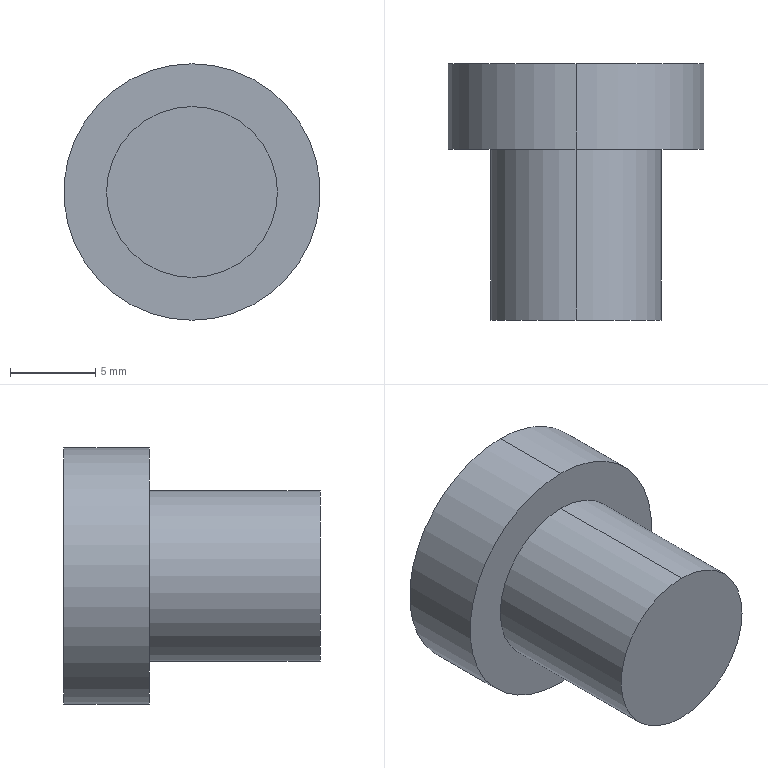Part | SolidWorks | features Extrusion 1, ICE 1 | 1 solid | 7 faces | box 15 x 15 x 15 mm | volume 1669 mm3 | cylinder 4 | plane 3 | commonest cylinder face diameters 10 x2 15 x2
STEP:
#1=CARTESIAN_POINT('',(0.,15.,7.5));
#2=VERTEX_POINT('',#1);
#3=CARTESIAN_POINT('',(0.,15.,-7.5));
#4=VERTEX_POINT('',#3);
#5=CARTESIAN_POINT('',(0.,15.,0.));
#6=DIRECTION('',(0.,1.,0.));
#7=DIRECTION('',(0.,0.,1.));
#8=AXIS2_PLACEMENT_3D('',#5,#6,#7);
#9=CIRCLE('',#8,7.5);
#10=EDGE_CURVE('',#2,#4,#9,.T.);
#11=ORIENTED_EDGE('',*,*,#10,.F.);
#12=CARTESIAN_POINT('',(0.,10.,7.5));
#13=VERTEX_POINT('',#12);
#14=CARTESIAN_POINT('',(0.,15.,7.5));
#15=DIRECTION('',(0.,-1.,0.));
#16=VECTOR('',#15,1000.);
#17=LINE('',#14,#16);
#18=EDGE_CURVE('',#2,#13,#17,.T.);
#19=ORIENTED_EDGE('',*,*,#18,.T.);
#20=CARTESIAN_POINT('',(0.,10.,-7.5));
#21=VERTEX_POINT('',#20);
#22=CARTESIAN_POINT('',(0.,10.,0.));
#23=DIRECTION('',(0.,1.,0.));
#24=DIRECTION('',(0.,0.,1.));
#25=AXIS2_PLACEMENT_3D('',#22,#23,#24);
#26=CIRCLE('',#25,7.5);
#27=EDGE_CURVE('',#13,#21,#26,.T.);
#28=ORIENTED_EDGE('',*,*,#27,.T.);
#29=CARTESIAN_POINT('',(0.,15.,-7.5));
#30=DIRECTION('',(0.,-1.,0.));
#31=VECTOR('',#30,1000.);
#32=LINE('',#29,#31);
#33=EDGE_CURVE('',#4,#21,#32,.T.);
#34=ORIENTED_EDGE('',*,*,#33,.F.);
#35=EDGE_LOOP('',(#11,#19,#28,#34));
#36=FACE_OUTER_BOUND('',#35,.T.);
#37=CARTESIAN_POINT('',(0.,15.,0.));
#38=DIRECTION('',(0.,-1.,0.));
#39=DIRECTION('',(0.,0.,-1.));
#40=AXIS2_PLACEMENT_3D('',#37,#38,#39);
#41=CYLINDRICAL_SURFACE('',#40,7.5);
#42=ADVANCED_FACE('',(#36),#41,.T.);
#43=CARTESIAN_POINT('',(0.,10.,5.));
#44=VERTEX_POINT('',#43);
#45=CARTESIAN_POINT('',(0.,10.,-5.));
#46=VERTEX_POINT('',#45);
#47=CARTESIAN_POINT('',(0.,10.,0.));
#48=DIRECTION('',(0.,1.,0.));
#49=DIRECTION('',(0.,0.,1.));
#50=AXIS2_PLACEMENT_3D('',#47,#48,#49);
#51=CIRCLE('',#50,5.);
#52=EDGE_CURVE('',#44,#46,#51,.T.);
#53=ORIENTED_EDGE('',*,*,#52,.F.);
#54=CARTESIAN_POINT('',(0.,0.,5.));
#55=VERTEX_POINT('',#54);
#56=CARTESIAN_POINT('',(0.,10.,5.));
#57=DIRECTION('',(0.,-1.,0.));
#58=VECTOR('',#57,1000.);
#59=LINE('',#56,#58);
#60=EDGE_CURVE('',#44,#55,#59,.T.);
#61=ORIENTED_EDGE('',*,*,#60,.T.);
#62=CARTESIAN_POINT('',(0.,0.,-5.));
#63=VERTEX_POINT('',#62);
#64=CARTESIAN_POINT('',(0.,0.,0.));
#65=DIRECTION('',(0.,1.,0.));
#66=DIRECTION('',(0.,0.,1.));
#67=AXIS2_PLACEMENT_3D('',#64,#65,#66);
#68=CIRCLE('',#67,5.);
#69=EDGE_CURVE('',#55,#63,#68,.T.);
#70=ORIENTED_EDGE('',*,*,#69,.T.);
#71=CARTESIAN_POINT('',(0.,10.,-5.));
#72=DIRECTION('',(0.,-1.,0.));
#73=VECTOR('',#72,1000.);
#74=LINE('',#71,#73);
#75=EDGE_CURVE('',#46,#63,#74,.T.);
#76=ORIENTED_EDGE('',*,*,#75,.F.);
#77=EDGE_LOOP('',(#53,#61,#70,#76));
#78=FACE_OUTER_BOUND('',#77,.T.);
#79=CARTESIAN_POINT('',(0.,10.,0.));
#80=DIRECTION('',(0.,-1.,0.));
#81=DIRECTION('',(0.,0.,-1.));
#82=AXIS2_PLACEMENT_3D('',#79,#80,#81);
#83=CYLINDRICAL_SURFACE('',#82,5.);
#84=ADVANCED_FACE('',(#78),#83,.T.);
#85=ORIENTED_EDGE('',*,*,#60,.F.);
#86=CARTESIAN_POINT('',(0.,10.,0.));
#87=DIRECTION('',(0.,1.,0.));
#88=DIRECTION('',(0.,0.,1.));
#89=AXIS2_PLACEMENT_3D('',#86,#87,#88);
#90=CIRCLE('',#89,5.);
#91=EDGE_CURVE('',#46,#44,#90,.T.);
#92=ORIENTED_EDGE('',*,*,#91,.F.);
#93=ORIENTED_EDGE('',*,*,#75,.T.);
#94=CARTESIAN_POINT('',(0.,0.,0.));
#95=DIRECTION('',(0.,1.,0.));
#96=DIRECTION('',(0.,0.,1.));
#97=AXIS2_PLACEMENT_3D('',#94,#95,#96);
#98=CIRCLE('',#97,5.);
#99=EDGE_CURVE('',#63,#55,#98,.T.);
#100=ORIENTED_EDGE('',*,*,#99,.T.);
#101=EDGE_LOOP('',(#85,#92,#93,#100));
#102=FACE_OUTER_BOUND('',#101,.T.);
#103=CARTESIAN_POINT('',(0.,10.,0.));
#104=DIRECTION('',(0.,-1.,0.));
#105=DIRECTION('',(0.,0.,-1.));
#106=AXIS2_PLACEMENT_3D('',#103,#104,#105);
#107=CYLINDRICAL_SURFACE('',#106,5.);
#108=ADVANCED_FACE('',(#102),#107,.T.);
#109=ORIENTED_EDGE('',*,*,#99,.F.);
#110=ORIENTED_EDGE('',*,*,#69,.F.);
#111=EDGE_LOOP('',(#109,#110));
#112=FACE_OUTER_BOUND('',#111,.T.);
#113=CARTESIAN_POINT('',(0.,0.,0.));
#114=DIRECTION('',(0.,1.,0.));
#115=DIRECTION('',(0.,0.,1.));
#116=AXIS2_PLACEMENT_3D('',#113,#114,#115);
#117=PLANE('',#116);
#118=ADVANCED_FACE('',(#112),#117,.F.);
#119=ORIENTED_EDGE('',*,*,#18,.F.);
#120=CARTESIAN_POINT('',(0.,15.,0.));
#121=DIRECTION('',(0.,1.,0.));
#122=DIRECTION('',(0.,0.,1.));
#123=AXIS2_PLACEMENT_3D('',#120,#121,#122);
#124=CIRCLE('',#123,7.5);
#125=EDGE_CURVE('',#4,#2,#124,.T.);
#126=ORIENTED_EDGE('',*,*,#125,.F.);
#127=ORIENTED_EDGE('',*,*,#33,.T.);
#128=CARTESIAN_POINT('',(0.,10.,0.));
#129=DIRECTION('',(0.,1.,0.));
#130=DIRECTION('',(0.,0.,1.));
#131=AXIS2_PLACEMENT_3D('',#128,#129,#130);
#132=CIRCLE('',#131,7.5);
#133=EDGE_CURVE('',#21,#13,#132,.T.);
#134=ORIENTED_EDGE('',*,*,#133,.T.);
#135=EDGE_LOOP('',(#119,#126,#127,#134));
#136=FACE_OUTER_BOUND('',#135,.T.);
#137=CARTESIAN_POINT('',(0.,15.,0.));
#138=DIRECTION('',(0.,-1.,0.));
#139=DIRECTION('',(0.,0.,-1.));
#140=AXIS2_PLACEMENT_3D('',#137,#138,#139);
#141=CYLINDRICAL_SURFACE('',#140,7.5);
#142=ADVANCED_FACE('',(#136),#141,.T.);
#143=ORIENTED_EDGE('',*,*,#125,.T.);
#144=ORIENTED_EDGE('',*,*,#10,.T.);
#145=EDGE_LOOP('',(#143,#144));
#146=FACE_OUTER_BOUND('',#145,.T.);
#147=CARTESIAN_POINT('',(0.,15.,0.));
#148=DIRECTION('',(0.,1.,0.));
#149=DIRECTION('',(0.,0.,1.));
#150=AXIS2_PLACEMENT_3D('',#147,#148,#149);
#151=PLANE('',#150);
#152=ADVANCED_FACE('',(#146),#151,.T.);
#153=ORIENTED_EDGE('',*,*,#91,.T.);
#154=ORIENTED_EDGE('',*,*,#52,.T.);
#155=EDGE_LOOP('',(#153,#154));
#156=FACE_BOUND('',#155,.T.);
#157=ORIENTED_EDGE('',*,*,#133,.F.);
#158=ORIENTED_EDGE('',*,*,#27,.F.);
#159=EDGE_LOOP('',(#157,#158));
#160=FACE_OUTER_BOUND('',#159,.T.);
#161=CARTESIAN_POINT('',(0.,10.,0.));
#162=DIRECTION('',(0.,1.,0.));
#163=DIRECTION('',(0.,0.,1.));
#164=AXIS2_PLACEMENT_3D('',#161,#162,#163);
#165=PLANE('',#164);
#166=ADVANCED_FACE('',(#156,#160),#165,.F.);
#167=CLOSED_SHELL('',(#42,#84,#108,#118,#142,#152,#166));
#168=MANIFOLD_SOLID_BREP('',#167);
#169=CARTESIAN_POINT('',(0.,0.,0.));
#170=DIRECTION('',(0.,0.,1.));
#171=DIRECTION('',(1.,0.,0.));
#172=AXIS2_PLACEMENT_3D('',#169,#170,#171);
#173=(LENGTH_UNIT()NAMED_UNIT(*)SI_UNIT(.MILLI.,.METRE.));
#174=UNCERTAINTY_MEASURE_WITH_UNIT(LENGTH_MEASURE(0.00001),#173,'','');
#175=(NAMED_UNIT(*)PLANE_ANGLE_UNIT()SI_UNIT($,.RADIAN.));
#176=(NAMED_UNIT(*)SI_UNIT($,.STERADIAN.)SOLID_ANGLE_UNIT());
#177=(GEOMETRIC_REPRESENTATION_CONTEXT(3)GLOBAL_UNCERTAINTY_ASSIGNED_CONTEXT((#174))GLOBAL_UNIT_ASSIGNED_CONTEXT((#173,#175,#176))REPRESENTATION_CONTEXT('',''));
#178=ADVANCED_BREP_SHAPE_REPRESENTATION('',(#168,#172),#177);